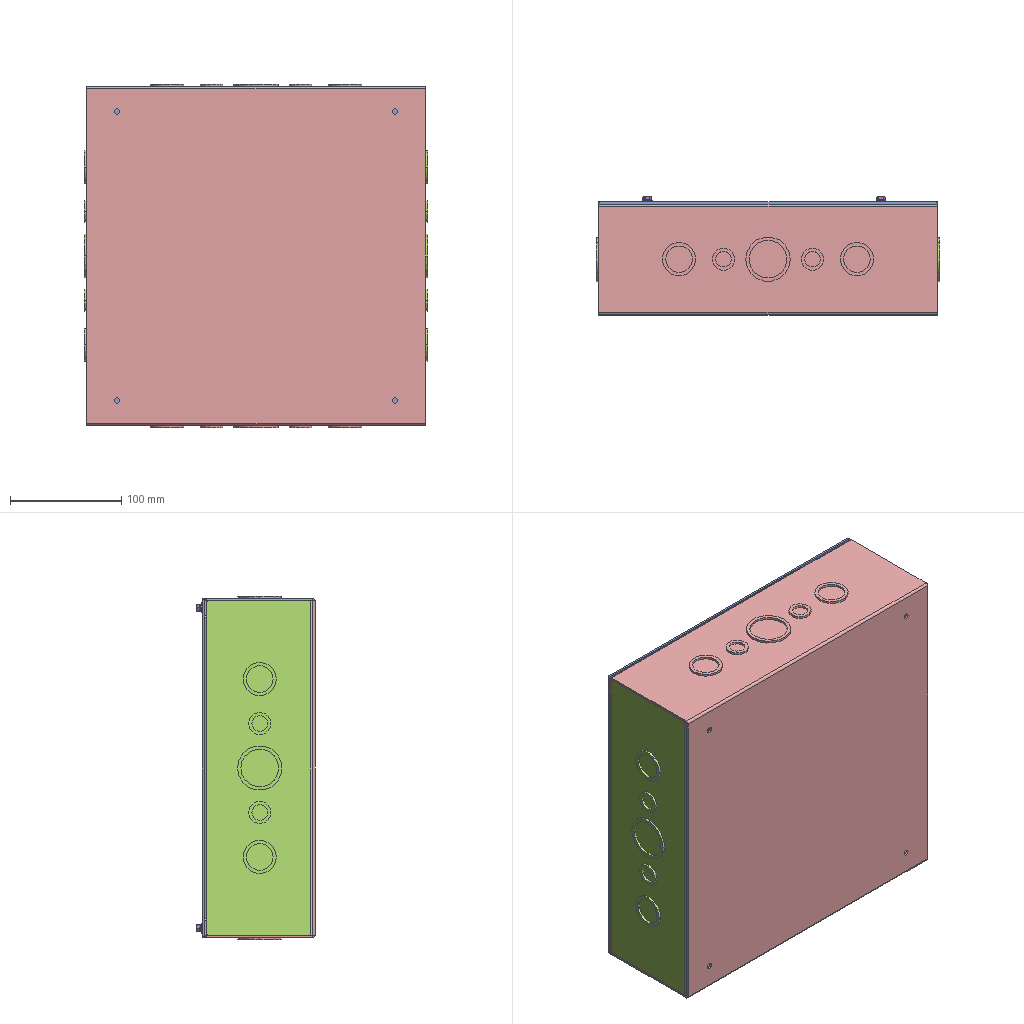Assembly | SolidWorks | 12 different items | 23 placed | box 309 x 106 x 309 mm
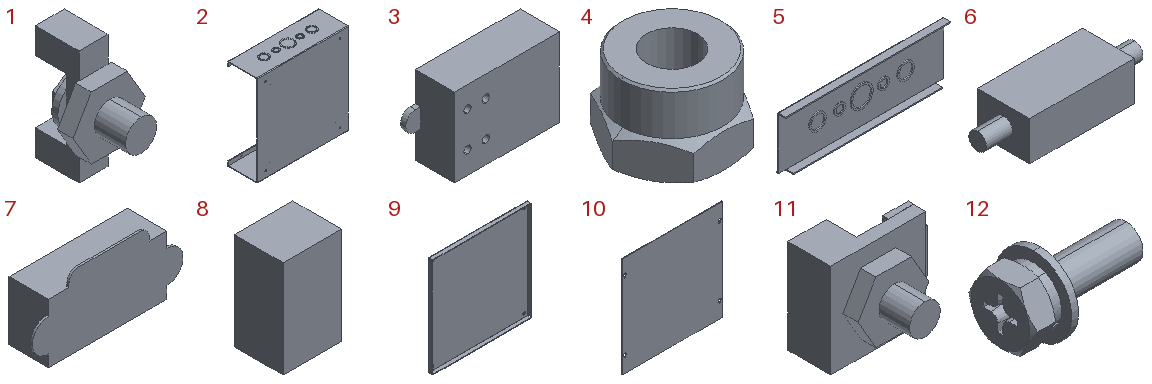Parts list (item | quantity | size | volume | features):
1 | x3 | 23.094 x 29 x 36.628 mm | 5934 mm3 | features ICE 7, Extrusion 1
2 | x1 | 304.8 x 99.6 x 308.8 mm | 331493 mm3 | features ICE 7, EdgeFlange 2, Cut 1, Fillet 1, FlatPattern 1, LPattern 1, SMBaseFlange 1, SheetMetal 1
3 | x1 | 51.375 x 15 x 30 mm | 18020 mm3 | features ICE 2, Extrusion 1
4 | x4 | 11.547 x 10 x 8 mm | 473.326 mm3 | features RevCut 3, Boss 1, Chamfer 1, Extrusion 1, LPattern 1
5 | x2 | 300.8 x 17 x 97.6 mm | 77629 mm3 | features EdgeFlange 2, ICE 2, Fillet 1, FlatPattern 1, SMBaseFlange 1, SheetMetal 1
6 | x1 | 42 x 14 x 10.5 mm | 3376 mm3 | features ICE 4, Extrusion 1, Scale 1
7 | x1 | 76.413 x 20 x 41.556 mm | 37640 mm3 | features ICE 2, Extrusion 1
8 | x1 | 60 x 50 x 100 mm | 300000 mm3 | features Extrusion 1
9 | x1 | 240.001 x 10 x 240.001 mm | 97684 mm3 | features EdgeFlange 1, FlatPattern 1, ICE 1, SMBaseFlange 1, SheetMetal 1
10 | x1 | 304.8 x 2 x 304.8 mm | 185210 mm3 | features Fillet 1, FlatPattern 1, ICE 1, LPattern 1, SMBaseFlange 1, SheetMetal 1
11 | x3 | 39.277 x 29 x 30.752 mm | 9979 mm3 | features ICE 9, Extrusion 1
12 | x4 | 14.8 x 9 x 9 mm | 319.757 mm3 | features BaseBody 3
Mates (type | each side: item.copy, entity, surface, feature):
Coincident | 2.1 plane | assembly plane | 3 times
Coincident | 2.1 face plane Edge-Flange1 | 10.1 face plane Base-Flange1 | 2 times
Coincident | 2.1 face plane Edge-Flange2 | 10.1 face plane Base-Flange1 | 2 times
Coincident | 2.1 face plane Base-Flange1 | 5.1 face plane Edge-Flange1
Coincident | 2.1 face plane Edge-Flange1 | 5.1 face plane Base-Flange1
Symmetric | 2.1 face plane Edge-Flange1 | 2.1 face plane Edge-Flange1 | 5.1 plane
Coincident | 2.1 face plane Edge-Flange1 | 5.2 face plane Base-Flange1
Coincident | 5.1 face plane Edge-Flange2 | 5.2 face plane Edge-Flange2
Coincident | 5.1 face plane Base-Flange1 | 5.2 face plane Base-Flange1
Symmetric | 2.1 face plane Edge-Flange1 | 2.1 face plane Edge-Flange1 | 9.1 plane
Symmetric | 5.1 face plane Base-Flange1 | 5.2 face plane Base-Flange1 | 9.1 plane
Coincident | 2.1 face plane Base-Flange1 | 9.1 face plane Edge-Flange1
Concentric | 9.1 face cylinder Cut-Extrude1 | 4.1 face cone EndChamfer
Coincident | 9.1 face plane Base-Flange1 | 4.1 face plane BaseNut
Concentric | 9.1 face cylinder Cut-Extrude1 | 4.2 face cone EndChamfer
Coincident | 9.1 face plane Base-Flange1 | 4.2 face plane BaseNut
Concentric | 2.1 face cylinder Boss-Extrude5 | 4.3 face cylinder Extrude1
Concentric | 9.1 face cylinder Cut-Extrude1 | 4.4 face cone EndChamfer
Coincident | 9.1 face plane Base-Flange1 | 4.4 face plane BaseNut
Coincident | 9.1 face plane Base-Flange1 | 4.3 face plane BaseNut
Coincident | 9.1 face plane Base-Flange1 | 1.1 face plane Boss-Extrude1
Parallel | 5.2 face plane Base-Flange1 | 1.1 face plane Boss-Extrude3
Coincident | 9.1 face plane Base-Flange1 | 11.1 face plane Boss-Extrude1
Parallel | 5.1 face plane Base-Flange1 | 11.1 face plane Boss-Extrude3
Coincident | 9.1 face plane Base-Flange1 | 6.1 face plane Boss-Extrude1
Coincident | 9.1 face plane Base-Flange1 | 7.1 face plane Boss-Extrude1
Parallel | 2.1 face plane Edge-Flange1 | 7.1 face plane Boss-Extrude1
Coincident | 9.1 face plane Base-Flange1 | 8.1 face plane Boss-Extrude1
Parallel | 2.1 face plane Edge-Flange1 | 8.1 face plane Boss-Extrude1
Coincident | 9.1 face plane Base-Flange1 | 3.1 face plane Boss-Extrude1
Concentric | 10.1 face cylinder LPattern1 | 12.1 face cylinder PN_0003 Plain washer grade A ∅4 stainless steel 304 GB.T 97.1-2002-2-solid1
Coincident | 10.1 face plane Base-Flange1 | 12.1 face plane PN_0003 Plain washer grade A ∅4 stainless steel 304 GB.T 97.1-2002-2-solid1
Concentric | 10.1 face cylinder Cut-Extrude1 | 12.2 face cylinder PN_0003 Plain washer grade A ∅4 stainless steel 304 GB.T 97.1-2002-2-solid1
Coincident | 10.1 face plane Base-Flange1 | 12.2 face plane PN_0003 Plain washer grade A ∅4 stainless steel 304 GB.T 97.1-2002-2-solid1
Concentric | 10.1 face cylinder Cut-Extrude1 | 12.3 face cylinder PN_0003 Plain washer grade A ∅4 stainless steel 304 GB.T 97.1-2002-2-solid1
Coincident | 10.1 face plane Base-Flange1 | 12.3 face plane PN_0003 Plain washer grade A ∅4 stainless steel 304 GB.T 97.1-2002-2-solid1
Concentric | 10.1 face cylinder LPattern1 | 12.4 face cylinder PN_0003 Plain washer grade A ∅4 stainless steel 304 GB.T 97.1-2002-2-solid1
Coincident | 10.1 face plane Base-Flange1 | 12.4 face plane PN_0003 Plain washer grade A ∅4 stainless steel 304 GB.T 97.1-2002-2-solid1